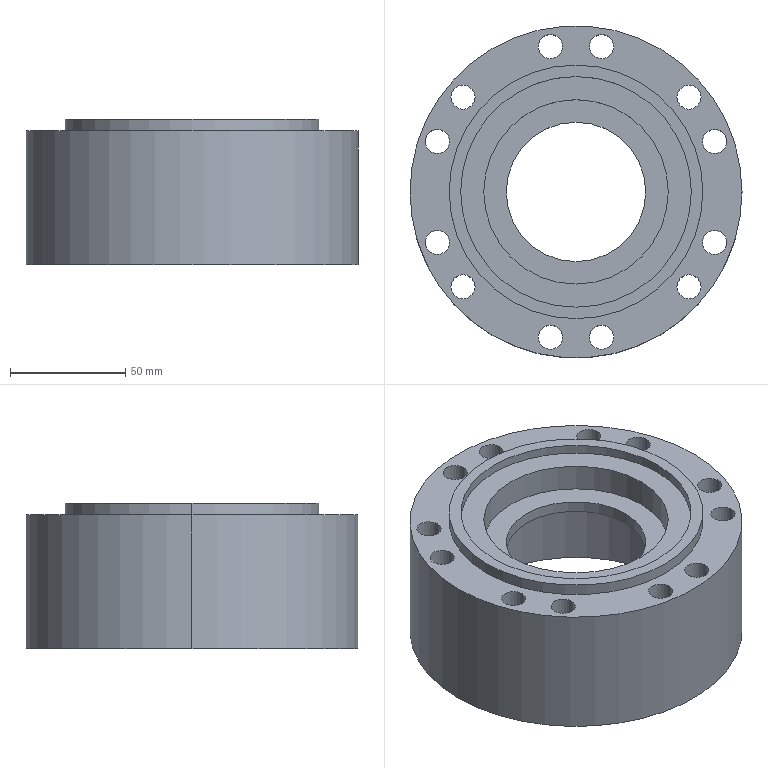Part | SolidWorks | features ICE 5, Extrusion 1, HoleWzd 1 | 1 solid | 42 faces | box 144 x 144 x 63 mm | volume 426591 mm3 | cylinder 36 | plane 6 | commonest cylinder face diameters 10.5 x24 110 x4 60.5 x2 80 x2 100 x2 144 x2
STEP:
#1=CARTESIAN_POINT('',(50.,0.,63.));
#2=VERTEX_POINT('',#1);
#3=CARTESIAN_POINT('',(-50.,0.,63.));
#4=VERTEX_POINT('',#3);
#5=CARTESIAN_POINT('',(0.,0.,63.));
#6=DIRECTION('',(0.,0.,-1.));
#7=DIRECTION('',(-1.,0.,0.));
#8=AXIS2_PLACEMENT_3D('',#5,#6,#7);
#9=CIRCLE('',#8,50.);
#10=EDGE_CURVE('',#2,#4,#9,.T.);
#11=ORIENTED_EDGE('',*,*,#10,.F.);
#12=CARTESIAN_POINT('',(50.,0.,59.));
#13=VERTEX_POINT('',#12);
#14=CARTESIAN_POINT('',(50.,0.,63.));
#15=DIRECTION('',(0.,0.,-1.));
#16=VECTOR('',#15,1000.);
#17=LINE('',#14,#16);
#18=EDGE_CURVE('',#2,#13,#17,.T.);
#19=ORIENTED_EDGE('',*,*,#18,.T.);
#20=CARTESIAN_POINT('',(-50.,0.,59.));
#21=VERTEX_POINT('',#20);
#22=CARTESIAN_POINT('',(0.,0.,59.));
#23=DIRECTION('',(0.,0.,-1.));
#24=DIRECTION('',(-1.,0.,0.));
#25=AXIS2_PLACEMENT_3D('',#22,#23,#24);
#26=CIRCLE('',#25,50.);
#27=EDGE_CURVE('',#13,#21,#26,.T.);
#28=ORIENTED_EDGE('',*,*,#27,.T.);
#29=CARTESIAN_POINT('',(-50.,0.,63.));
#30=DIRECTION('',(0.,0.,-1.));
#31=VECTOR('',#30,1000.);
#32=LINE('',#29,#31);
#33=EDGE_CURVE('',#4,#21,#32,.T.);
#34=ORIENTED_EDGE('',*,*,#33,.F.);
#35=EDGE_LOOP('',(#11,#19,#28,#34));
#36=FACE_OUTER_BOUND('',#35,.T.);
#37=CARTESIAN_POINT('',(0.,0.,63.));
#38=DIRECTION('',(0.,0.,-1.));
#39=DIRECTION('',(-1.,0.,0.));
#40=AXIS2_PLACEMENT_3D('',#37,#38,#39);
#41=CYLINDRICAL_SURFACE('',#40,50.);
#42=ADVANCED_FACE('',(#36),#41,.F.);
#43=CARTESIAN_POINT('',(-40.,0.,59.));
#44=VERTEX_POINT('',#43);
#45=CARTESIAN_POINT('',(40.,0.,59.));
#46=VERTEX_POINT('',#45);
#47=CARTESIAN_POINT('',(0.,0.,59.));
#48=DIRECTION('',(0.,0.,1.));
#49=DIRECTION('',(-1.,0.,0.));
#50=AXIS2_PLACEMENT_3D('',#47,#48,#49);
#51=CIRCLE('',#50,40.);
#52=EDGE_CURVE('',#44,#46,#51,.T.);
#53=ORIENTED_EDGE('',*,*,#52,.T.);
#54=CARTESIAN_POINT('',(40.,0.,47.));
#55=VERTEX_POINT('',#54);
#56=CARTESIAN_POINT('',(40.,0.,59.));
#57=DIRECTION('',(0.,0.,-1.));
#58=VECTOR('',#57,1000.);
#59=LINE('',#56,#58);
#60=EDGE_CURVE('',#46,#55,#59,.T.);
#61=ORIENTED_EDGE('',*,*,#60,.T.);
#62=CARTESIAN_POINT('',(-40.,0.,47.));
#63=VERTEX_POINT('',#62);
#64=CARTESIAN_POINT('',(0.,0.,47.));
#65=DIRECTION('',(0.,0.,-1.));
#66=DIRECTION('',(-1.,0.,0.));
#67=AXIS2_PLACEMENT_3D('',#64,#65,#66);
#68=CIRCLE('',#67,40.);
#69=EDGE_CURVE('',#55,#63,#68,.T.);
#70=ORIENTED_EDGE('',*,*,#69,.T.);
#71=CARTESIAN_POINT('',(-40.,0.,59.));
#72=DIRECTION('',(0.,0.,-1.));
#73=VECTOR('',#72,1000.);
#74=LINE('',#71,#73);
#75=EDGE_CURVE('',#44,#63,#74,.T.);
#76=ORIENTED_EDGE('',*,*,#75,.F.);
#77=EDGE_LOOP('',(#53,#61,#70,#76));
#78=FACE_OUTER_BOUND('',#77,.T.);
#79=CARTESIAN_POINT('',(0.,0.,59.));
#80=DIRECTION('',(0.,0.,-1.));
#81=DIRECTION('',(-1.,0.,0.));
#82=AXIS2_PLACEMENT_3D('',#79,#80,#81);
#83=CYLINDRICAL_SURFACE('',#82,40.);
#84=ADVANCED_FACE('',(#78),#83,.F.);
#85=CARTESIAN_POINT('',(-30.25,0.,47.));
#86=VERTEX_POINT('',#85);
#87=CARTESIAN_POINT('',(30.25,0.,47.));
#88=VERTEX_POINT('',#87);
#89=CARTESIAN_POINT('',(0.,0.,47.));
#90=DIRECTION('',(0.,0.,1.));
#91=DIRECTION('',(-1.,0.,0.));
#92=AXIS2_PLACEMENT_3D('',#89,#90,#91);
#93=CIRCLE('',#92,30.25);
#94=EDGE_CURVE('',#86,#88,#93,.T.);
#95=ORIENTED_EDGE('',*,*,#94,.T.);
#96=CARTESIAN_POINT('',(30.25,0.,42.));
#97=VERTEX_POINT('',#96);
#98=CARTESIAN_POINT('',(30.25,0.,47.));
#99=DIRECTION('',(0.,0.,-1.));
#100=VECTOR('',#99,1000.);
#101=LINE('',#98,#100);
#102=EDGE_CURVE('',#88,#97,#101,.T.);
#103=ORIENTED_EDGE('',*,*,#102,.T.);
#104=CARTESIAN_POINT('',(-30.25,0.,42.));
#105=VERTEX_POINT('',#104);
#106=CARTESIAN_POINT('',(0.,0.,42.));
#107=DIRECTION('',(0.,0.,-1.));
#108=DIRECTION('',(-1.,0.,0.));
#109=AXIS2_PLACEMENT_3D('',#106,#107,#108);
#110=CIRCLE('',#109,30.25);
#111=EDGE_CURVE('',#97,#105,#110,.T.);
#112=ORIENTED_EDGE('',*,*,#111,.T.);
#113=CARTESIAN_POINT('',(-30.25,0.,47.));
#114=DIRECTION('',(0.,0.,-1.));
#115=VECTOR('',#114,1000.);
#116=LINE('',#113,#115);
#117=EDGE_CURVE('',#86,#105,#116,.T.);
#118=ORIENTED_EDGE('',*,*,#117,.F.);
#119=EDGE_LOOP('',(#95,#103,#112,#118));
#120=FACE_OUTER_BOUND('',#119,.T.);
#121=CARTESIAN_POINT('',(0.,0.,47.));
#122=DIRECTION('',(0.,0.,-1.));
#123=DIRECTION('',(-1.,0.,0.));
#124=AXIS2_PLACEMENT_3D('',#121,#122,#123);
#125=CYLINDRICAL_SURFACE('',#124,30.25);
#126=ADVANCED_FACE('',(#120),#125,.F.);
#127=CARTESIAN_POINT('',(55.,0.,42.));
#128=VERTEX_POINT('',#127);
#129=CARTESIAN_POINT('',(-55.,0.,42.));
#130=VERTEX_POINT('',#129);
#131=CARTESIAN_POINT('',(0.,0.,42.));
#132=DIRECTION('',(0.,0.,-1.));
#133=DIRECTION('',(-1.,0.,0.));
#134=AXIS2_PLACEMENT_3D('',#131,#132,#133);
#135=CIRCLE('',#134,55.);
#136=EDGE_CURVE('',#128,#130,#135,.T.);
#137=ORIENTED_EDGE('',*,*,#136,.F.);
#138=CARTESIAN_POINT('',(55.,0.,0.));
#139=VERTEX_POINT('',#138);
#140=CARTESIAN_POINT('',(55.,0.,42.));
#141=DIRECTION('',(0.,0.,-1.));
#142=VECTOR('',#141,1000.);
#143=LINE('',#140,#142);
#144=EDGE_CURVE('',#128,#139,#143,.T.);
#145=ORIENTED_EDGE('',*,*,#144,.T.);
#146=CARTESIAN_POINT('',(-55.,0.,0.));
#147=VERTEX_POINT('',#146);
#148=CARTESIAN_POINT('',(0.,0.,0.));
#149=DIRECTION('',(0.,0.,-1.));
#150=DIRECTION('',(-1.,0.,0.));
#151=AXIS2_PLACEMENT_3D('',#148,#149,#150);
#152=CIRCLE('',#151,55.);
#153=EDGE_CURVE('',#139,#147,#152,.T.);
#154=ORIENTED_EDGE('',*,*,#153,.T.);
#155=CARTESIAN_POINT('',(-55.,0.,42.));
#156=DIRECTION('',(0.,0.,-1.));
#157=VECTOR('',#156,1000.);
#158=LINE('',#155,#157);
#159=EDGE_CURVE('',#130,#147,#158,.T.);
#160=ORIENTED_EDGE('',*,*,#159,.F.);
#161=EDGE_LOOP('',(#137,#145,#154,#160));
#162=FACE_OUTER_BOUND('',#161,.T.);
#163=CARTESIAN_POINT('',(0.,0.,42.));
#164=DIRECTION('',(0.,0.,-1.));
#165=DIRECTION('',(-1.,0.,0.));
#166=AXIS2_PLACEMENT_3D('',#163,#164,#165);
#167=CYLINDRICAL_SURFACE('',#166,55.);
#168=ADVANCED_FACE('',(#162),#167,.F.);
#169=CARTESIAN_POINT('',(5.863,63.028,58.));
#170=VERTEX_POINT('',#169);
#171=CARTESIAN_POINT('',(16.363,63.028,58.));
#172=VERTEX_POINT('',#171);
#173=CARTESIAN_POINT('',(11.113,63.028,58.));
#174=DIRECTION('',(0.,0.,1.));
#175=DIRECTION('',(1.,0.,0.));
#176=AXIS2_PLACEMENT_3D('',#173,#174,#175);
#177=CIRCLE('',#176,5.25);
#178=EDGE_CURVE('',#170,#172,#177,.T.);
#179=ORIENTED_EDGE('',*,*,#178,.T.);
#180=CARTESIAN_POINT('',(16.363,63.028,0.));
#181=VERTEX_POINT('',#180);
#182=CARTESIAN_POINT('',(16.363,63.028,0.));
#183=DIRECTION('',(0.,0.,-1.));
#184=VECTOR('',#183,1000.);
#185=LINE('',#182,#184);
#186=EDGE_CURVE('',#172,#181,#185,.T.);
#187=ORIENTED_EDGE('',*,*,#186,.T.);
#188=CARTESIAN_POINT('',(5.863,63.028,0.));
#189=VERTEX_POINT('',#188);
#190=CARTESIAN_POINT('',(11.113,63.028,0.));
#191=DIRECTION('',(0.,0.,-1.));
#192=DIRECTION('',(-1.,0.,0.));
#193=AXIS2_PLACEMENT_3D('',#190,#191,#192);
#194=CIRCLE('',#193,5.25);
#195=EDGE_CURVE('',#181,#189,#194,.T.);
#196=ORIENTED_EDGE('',*,*,#195,.T.);
#197=CARTESIAN_POINT('',(5.863,63.028,0.));
#198=DIRECTION('',(0.,0.,-1.));
#199=VECTOR('',#198,1000.);
#200=LINE('',#197,#199);
#201=EDGE_CURVE('',#170,#189,#200,.T.);
#202=ORIENTED_EDGE('',*,*,#201,.F.);
#203=EDGE_LOOP('',(#179,#187,#196,#202));
#204=FACE_OUTER_BOUND('',#203,.T.);
#205=CARTESIAN_POINT('',(11.113,63.028,0.));
#206=DIRECTION('',(0.,0.,-1.));
#207=DIRECTION('',(-1.,0.,0.));
#208=AXIS2_PLACEMENT_3D('',#205,#206,#207);
#209=CYLINDRICAL_SURFACE('',#208,5.25);
#210=ADVANCED_FACE('',(#204),#209,.F.);
#211=CARTESIAN_POINT('',(-16.363,63.028,58.));
#212=VERTEX_POINT('',#211);
#213=CARTESIAN_POINT('',(-5.863,63.028,58.));
#214=VERTEX_POINT('',#213);
#215=CARTESIAN_POINT('',(-11.113,63.028,58.));
#216=DIRECTION('',(0.,0.,1.));
#217=DIRECTION('',(1.,0.,0.));
#218=AXIS2_PLACEMENT_3D('',#215,#216,#217);
#219=CIRCLE('',#218,5.25);
#220=EDGE_CURVE('',#212,#214,#219,.T.);
#221=ORIENTED_EDGE('',*,*,#220,.T.);
#222=CARTESIAN_POINT('',(-5.863,63.028,0.));
#223=VERTEX_POINT('',#222);
#224=CARTESIAN_POINT('',(-5.863,63.028,0.));
#225=DIRECTION('',(0.,0.,-1.));
#226=VECTOR('',#225,1000.);
#227=LINE('',#224,#226);
#228=EDGE_CURVE('',#214,#223,#227,.T.);
#229=ORIENTED_EDGE('',*,*,#228,.T.);
#230=CARTESIAN_POINT('',(-16.363,63.028,0.));
#231=VERTEX_POINT('',#230);
#232=CARTESIAN_POINT('',(-11.113,63.028,0.));
#233=DIRECTION('',(0.,0.,-1.));
#234=DIRECTION('',(-1.,0.,0.));
#235=AXIS2_PLACEMENT_3D('',#232,#233,#234);
#236=CIRCLE('',#235,5.25);
#237=EDGE_CURVE('',#223,#231,#236,.T.);
#238=ORIENTED_EDGE('',*,*,#237,.T.);
#239=CARTESIAN_POINT('',(-16.363,63.028,0.));
#240=DIRECTION('',(0.,0.,-1.));
#241=VECTOR('',#240,1000.);
#242=LINE('',#239,#241);
#243=EDGE_CURVE('',#212,#231,#242,.T.);
#244=ORIENTED_EDGE('',*,*,#243,.F.);
#245=EDGE_LOOP('',(#221,#229,#238,#244));
#246=FACE_OUTER_BOUND('',#245,.T.);
#247=CARTESIAN_POINT('',(-11.113,63.028,0.));
#248=DIRECTION('',(0.,0.,-1.));
#249=DIRECTION('',(-1.,0.,0.));
#250=AXIS2_PLACEMENT_3D('',#247,#248,#249);
#251=CYLINDRICAL_SURFACE('',#250,5.25);
#252=ADVANCED_FACE('',(#246),#251,.F.);
#253=CARTESIAN_POINT('',(-54.277,41.138,58.));
#254=VERTEX_POINT('',#253);
#255=CARTESIAN_POINT('',(-43.777,41.138,58.));
#256=VERTEX_POINT('',#255);
#257=CARTESIAN_POINT('',(-49.027,41.138,58.));
#258=DIRECTION('',(0.,0.,1.));
#259=DIRECTION('',(1.,0.,0.));
#260=AXIS2_PLACEMENT_3D('',#257,#258,#259);
#261=CIRCLE('',#260,5.25);
#262=EDGE_CURVE('',#254,#256,#261,.T.);
#263=ORIENTED_EDGE('',*,*,#262,.T.);
#264=CARTESIAN_POINT('',(-43.777,41.138,0.));
#265=VERTEX_POINT('',#264);
#266=CARTESIAN_POINT('',(-43.777,41.138,0.));
#267=DIRECTION('',(0.,0.,-1.));
#268=VECTOR('',#267,1000.);
#269=LINE('',#266,#268);
#270=EDGE_CURVE('',#256,#265,#269,.T.);
#271=ORIENTED_EDGE('',*,*,#270,.T.);
#272=CARTESIAN_POINT('',(-54.277,41.138,0.));
#273=VERTEX_POINT('',#272);
#274=CARTESIAN_POINT('',(-49.027,41.138,0.));
#275=DIRECTION('',(0.,0.,-1.));
#276=DIRECTION('',(-1.,0.,0.));
#277=AXIS2_PLACEMENT_3D('',#274,#275,#276);
#278=CIRCLE('',#277,5.25);
#279=EDGE_CURVE('',#265,#273,#278,.T.);
#280=ORIENTED_EDGE('',*,*,#279,.T.);
#281=CARTESIAN_POINT('',(-54.277,41.138,0.));
#282=DIRECTION('',(0.,0.,-1.));
#283=VECTOR('',#282,1000.);
#284=LINE('',#281,#283);
#285=EDGE_CURVE('',#254,#273,#284,.T.);
#286=ORIENTED_EDGE('',*,*,#285,.F.);
#287=EDGE_LOOP('',(#263,#271,#280,#286));
#288=FACE_OUTER_BOUND('',#287,.T.);
#289=CARTESIAN_POINT('',(-49.027,41.138,0.));
#290=DIRECTION('',(0.,0.,-1.));
#291=DIRECTION('',(-1.,0.,0.));
#292=AXIS2_PLACEMENT_3D('',#289,#290,#291);
#293=CYLINDRICAL_SURFACE('',#292,5.25);
#294=ADVANCED_FACE('',(#288),#293,.F.);
#295=CARTESIAN_POINT('',(-65.39,21.889,58.));
#296=VERTEX_POINT('',#295);
#297=CARTESIAN_POINT('',(-54.89,21.889,58.));
#298=VERTEX_POINT('',#297);
#299=CARTESIAN_POINT('',(-60.14,21.889,58.));
#300=DIRECTION('',(0.,0.,1.));
#301=DIRECTION('',(1.,0.,0.));
#302=AXIS2_PLACEMENT_3D('',#299,#300,#301);
#303=CIRCLE('',#302,5.25);
#304=EDGE_CURVE('',#296,#298,#303,.T.);
#305=ORIENTED_EDGE('',*,*,#304,.T.);
#306=CARTESIAN_POINT('',(-54.89,21.889,0.));
#307=VERTEX_POINT('',#306);
#308=CARTESIAN_POINT('',(-54.89,21.889,0.));
#309=DIRECTION('',(0.,0.,-1.));
#310=VECTOR('',#309,1000.);
#311=LINE('',#308,#310);
#312=EDGE_CURVE('',#298,#307,#311,.T.);
#313=ORIENTED_EDGE('',*,*,#312,.T.);
#314=CARTESIAN_POINT('',(-65.39,21.889,0.));
#315=VERTEX_POINT('',#314);
#316=CARTESIAN_POINT('',(-60.14,21.889,0.));
#317=DIRECTION('',(0.,0.,-1.));
#318=DIRECTION('',(-1.,0.,0.));
#319=AXIS2_PLACEMENT_3D('',#316,#317,#318);
#320=CIRCLE('',#319,5.25);
#321=EDGE_CURVE('',#307,#315,#320,.T.);
#322=ORIENTED_EDGE('',*,*,#321,.T.);
#323=CARTESIAN_POINT('',(-65.39,21.889,0.));
#324=DIRECTION('',(0.,0.,-1.));
#325=VECTOR('',#324,1000.);
#326=LINE('',#323,#325);
#327=EDGE_CURVE('',#296,#315,#326,.T.);
#328=ORIENTED_EDGE('',*,*,#327,.F.);
#329=EDGE_LOOP('',(#305,#313,#322,#328));
#330=FACE_OUTER_BOUND('',#329,.T.);
#331=CARTESIAN_POINT('',(-60.14,21.889,0.));
#332=DIRECTION('',(0.,0.,-1.));
#333=DIRECTION('',(-1.,0.,0.));
#334=AXIS2_PLACEMENT_3D('',#331,#332,#333);
#335=CYLINDRICAL_SURFACE('',#334,5.25);
#336=ADVANCED_FACE('',(#330),#335,.F.);
#337=CARTESIAN_POINT('',(-65.39,-21.889,58.));
#338=VERTEX_POINT('',#337);
#339=CARTESIAN_POINT('',(-54.89,-21.889,58.));
#340=VERTEX_POINT('',#339);
#341=CARTESIAN_POINT('',(-60.14,-21.889,58.));
#342=DIRECTION('',(0.,0.,1.));
#343=DIRECTION('',(1.,0.,0.));
#344=AXIS2_PLACEMENT_3D('',#341,#342,#343);
#345=CIRCLE('',#344,5.25);
#346=EDGE_CURVE('',#338,#340,#345,.T.);
#347=ORIENTED_EDGE('',*,*,#346,.T.);
#348=CARTESIAN_POINT('',(-54.89,-21.889,0.));
#349=VERTEX_POINT('',#348);
#350=CARTESIAN_POINT('',(-54.89,-21.889,0.));
#351=DIRECTION('',(0.,0.,-1.));
#352=VECTOR('',#351,1000.);
#353=LINE('',#350,#352);
#354=EDGE_CURVE('',#340,#349,#353,.T.);
#355=ORIENTED_EDGE('',*,*,#354,.T.);
#356=CARTESIAN_POINT('',(-65.39,-21.889,0.));
#357=VERTEX_POINT('',#356);
#358=CARTESIAN_POINT('',(-60.14,-21.889,0.));
#359=DIRECTION('',(0.,0.,-1.));
#360=DIRECTION('',(-1.,0.,0.));
#361=AXIS2_PLACEMENT_3D('',#358,#359,#360);
#362=CIRCLE('',#361,5.25);
#363=EDGE_CURVE('',#349,#357,#362,.T.);
#364=ORIENTED_EDGE('',*,*,#363,.T.);
#365=CARTESIAN_POINT('',(-65.39,-21.889,0.));
#366=DIRECTION('',(0.,0.,-1.));
#367=VECTOR('',#366,1000.);
#368=LINE('',#365,#367);
#369=EDGE_CURVE('',#338,#357,#368,.T.);
#370=ORIENTED_EDGE('',*,*,#369,.F.);
#371=EDGE_LOOP('',(#347,#355,#364,#370));
#372=FACE_OUTER_BOUND('',#371,.T.);
#373=CARTESIAN_POINT('',(-60.14,-21.889,0.));
#374=DIRECTION('',(0.,0.,-1.));
#375=DIRECTION('',(-1.,0.,0.));
#376=AXIS2_PLACEMENT_3D('',#373,#374,#375);
#377=CYLINDRICAL_SURFACE('',#376,5.25);
#378=ADVANCED_FACE('',(#372),#377,.F.);
#379=CARTESIAN_POINT('',(-54.277,-41.138,58.));
#380=VERTEX_POINT('',#379);
#381=CARTESIAN_POINT('',(-43.777,-41.138,58.));
#382=VERTEX_POINT('',#381);
#383=CARTESIAN_POINT('',(-49.027,-41.138,58.));
#384=DIRECTION('',(0.,0.,1.));
#385=DIRECTION('',(1.,0.,0.));
#386=AXIS2_PLACEMENT_3D('',#383,#384,#385);
#387=CIRCLE('',#386,5.25);
#388=EDGE_CURVE('',#380,#382,#387,.T.);
#389=ORIENTED_EDGE('',*,*,#388,.T.);
#390=CARTESIAN_POINT('',(-43.777,-41.138,0.));
#391=VERTEX_POINT('',#390);
#392=CARTESIAN_POINT('',(-43.777,-41.138,0.));
#393=DIRECTION('',(0.,0.,-1.));
#394=VECTOR('',#393,1000.);
#395=LINE('',#392,#394);
#396=EDGE_CURVE('',#382,#391,#395,.T.);
#397=ORIENTED_EDGE('',*,*,#396,.T.);
#398=CARTESIAN_POINT('',(-54.277,-41.138,0.));
#399=VERTEX_POINT('',#398);
#400=CARTESIAN_POINT('',(-49.027,-41.138,0.));
#401=DIRECTION('',(0.,0.,-1.));
#402=DIRECTION('',(-1.,0.,0.));
#403=AXIS2_PLACEMENT_3D('',#400,#401,#402);
#404=CIRCLE('',#403,5.25);
#405=EDGE_CURVE('',#391,#399,#404,.T.);
#406=ORIENTED_EDGE('',*,*,#405,.T.);
#407=CARTESIAN_POINT('',(-54.277,-41.138,0.));
#408=DIRECTION('',(0.,0.,-1.));
#409=VECTOR('',#408,1000.);
#410=LINE('',#407,#409);
#411=EDGE_CURVE('',#380,#399,#410,.T.);
#412=ORIENTED_EDGE('',*,*,#411,.F.);
#413=EDGE_LOOP('',(#389,#397,#406,#412));
#414=FACE_OUTER_BOUND('',#413,.T.);
#415=CARTESIAN_POINT('',(-49.027,-41.138,0.));
#416=DIRECTION('',(0.,0.,-1.));
#417=DIRECTION('',(-1.,0.,0.));
#418=AXIS2_PLACEMENT_3D('',#415,#416,#417);
#419=CYLINDRICAL_SURFACE('',#418,5.25);
#420=ADVANCED_FACE('',(#414),#419,.F.);
#421=CARTESIAN_POINT('',(-16.363,-63.028,58.));
#422=VERTEX_POINT('',#421);
#423=CARTESIAN_POINT('',(-5.863,-63.028,58.));
#424=VERTEX_POINT('',#423);
#425=CARTESIAN_POINT('',(-11.113,-63.028,58.));
#426=DIRECTION('',(0.,0.,1.));
#427=DIRECTION('',(1.,0.,0.));
#428=AXIS2_PLACEMENT_3D('',#425,#426,#427);
#429=CIRCLE('',#428,5.25);
#430=EDGE_CURVE('',#422,#424,#429,.T.);
#431=ORIENTED_EDGE('',*,*,#430,.T.);
#432=CARTESIAN_POINT('',(-5.863,-63.028,0.));
#433=VERTEX_POINT('',#432);
#434=CARTESIAN_POINT('',(-5.863,-63.028,0.));
#435=DIRECTION('',(0.,0.,-1.));
#436=VECTOR('',#435,1000.);
#437=LINE('',#434,#436);
#438=EDGE_CURVE('',#424,#433,#437,.T.);
#439=ORIENTED_EDGE('',*,*,#438,.T.);
#440=CARTESIAN_POINT('',(-16.363,-63.028,0.));
#441=VERTEX_POINT('',#440);
#442=CARTESIAN_POINT('',(-11.113,-63.028,0.));
#443=DIRECTION('',(0.,0.,-1.));
#444=DIRECTION('',(-1.,0.,0.));
#445=AXIS2_PLACEMENT_3D('',#442,#443,#444);
#446=CIRCLE('',#445,5.25);
#447=EDGE_CURVE('',#433,#441,#446,.T.);
#448=ORIENTED_EDGE('',*,*,#447,.T.);
#449=CARTESIAN_POINT('',(-16.363,-63.028,0.));
#450=DIRECTION('',(0.,0.,-1.));
#451=VECTOR('',#450,1000.);
#452=LINE('',#449,#451);
#453=EDGE_CURVE('',#422,#441,#452,.T.);
#454=ORIENTED_EDGE('',*,*,#453,.F.);
#455=EDGE_LOOP('',(#431,#439,#448,#454));
#456=FACE_OUTER_BOUND('',#455,.T.);
#457=CARTESIAN_POINT('',(-11.113,-63.028,0.));
#458=DIRECTION('',(0.,0.,-1.));
#459=DIRECTION('',(-1.,0.,0.));
#460=AXIS2_PLACEMENT_3D('',#457,#458,#459);
#461=CYLINDRICAL_SURFACE('',#460,5.25);
#462=ADVANCED_FACE('',(#456),#461,.F.);
#463=CARTESIAN_POINT('',(5.863,-63.028,58.));
#464=VERTEX_POINT('',#463);
#465=CARTESIAN_POINT('',(16.363,-63.028,58.));
#466=VERTEX_POINT('',#465);
#467=CARTESIAN_POINT('',(11.113,-63.028,58.));
#468=DIRECTION('',(0.,0.,1.));
#469=DIRECTION('',(1.,0.,0.));
#470=AXIS2_PLACEMENT_3D('',#467,#468,#469);
#471=CIRCLE('',#470,5.25);
#472=EDGE_CURVE('',#464,#466,#471,.T.);
#473=ORIENTED_EDGE('',*,*,#472,.T.);
#474=CARTESIAN_POINT('',(16.363,-63.028,0.));
#475=VERTEX_POINT('',#474);
#476=CARTESIAN_POINT('',(16.363,-63.028,0.));
#477=DIRECTION('',(0.,0.,-1.));
#478=VECTOR('',#477,1000.);
#479=LINE('',#476,#478);
#480=EDGE_CURVE('',#466,#475,#479,.T.);
#481=ORIENTED_EDGE('',*,*,#480,.T.);
#482=CARTESIAN_POINT('',(5.863,-63.028,0.));
#483=VERTEX_POINT('',#482);
#484=CARTESIAN_POINT('',(11.113,-63.028,0.));
#485=DIRECTION('',(0.,0.,-1.));
#486=DIRECTION('',(-1.,0.,0.));
#487=AXIS2_PLACEMENT_3D('',#484,#485,#486);
#488=CIRCLE('',#487,5.25);
#489=EDGE_CURVE('',#475,#483,#488,.T.);
#490=ORIENTED_EDGE('',*,*,#489,.T.);
#491=CARTESIAN_POINT('',(5.863,-63.028,0.));
#492=DIRECTION('',(0.,0.,-1.));
#493=VECTOR('',#492,1000.);
#494=LINE('',#491,#493);
#495=EDGE_CURVE('',#464,#483,#494,.T.);
#496=ORIENTED_EDGE('',*,*,#495,.F.);
#497=EDGE_LOOP('',(#473,#481,#490,#496));
#498=FACE_OUTER_BOUND('',#497,.T.);
#499=CARTESIAN_POINT('',(11.113,-63.028,0.));
#500=DIRECTION('',(0.,0.,-1.));
#501=DIRECTION('',(-1.,0.,0.));
#502=AXIS2_PLACEMENT_3D('',#499,#500,#501);
#503=CYLINDRICAL_SURFACE('',#502,5.25);
#504=ADVANCED_FACE('',(#498),#503,.F.);
#505=CARTESIAN_POINT('',(43.777,-41.138,58.));
#506=VERTEX_POINT('',#505);
#507=CARTESIAN_POINT('',(54.277,-41.138,58.));
#508=VERTEX_POINT('',#507);
#509=CARTESIAN_POINT('',(49.027,-41.138,58.));
#510=DIRECTION('',(0.,0.,1.));
#511=DIRECTION('',(1.,0.,0.));
#512=AXIS2_PLACEMENT_3D('',#509,#510,#511);
#513=CIRCLE('',#512,5.25);
#514=EDGE_CURVE('',#506,#508,#513,.T.);
#515=ORIENTED_EDGE('',*,*,#514,.T.);
#516=CARTESIAN_POINT('',(54.277,-41.138,0.));
#517=VERTEX_POINT('',#516);
#518=CARTESIAN_POINT('',(54.277,-41.138,0.));
#519=DIRECTION('',(0.,0.,-1.));
#520=VECTOR('',#519,1000.);
#521=LINE('',#518,#520);
#522=EDGE_CURVE('',#508,#517,#521,.T.);
#523=ORIENTED_EDGE('',*,*,#522,.T.);
#524=CARTESIAN_POINT('',(43.777,-41.138,0.));
#525=VERTEX_POINT('',#524);
#526=CARTESIAN_POINT('',(49.027,-41.138,0.));
#527=DIRECTION('',(0.,0.,-1.));
#528=DIRECTION('',(-1.,0.,0.));
#529=AXIS2_PLACEMENT_3D('',#526,#527,#528);
#530=CIRCLE('',#529,5.25);
#531=EDGE_CURVE('',#517,#525,#530,.T.);
#532=ORIENTED_EDGE('',*,*,#531,.T.);
#533=CARTESIAN_POINT('',(43.777,-41.138,0.));
#534=DIRECTION('',(0.,0.,-1.));
#535=VECTOR('',#534,1000.);
#536=LINE('',#533,#535);
#537=EDGE_CURVE('',#506,#525,#536,.T.);
#538=ORIENTED_EDGE('',*,*,#537,.F.);
#539=EDGE_LOOP('',(#515,#523,#532,#538));
#540=FACE_OUTER_BOUND('',#539,.T.);
#541=CARTESIAN_POINT('',(49.027,-41.138,0.));
#542=DIRECTION('',(0.,0.,-1.));
#543=DIRECTION('',(-1.,0.,0.));
#544=AXIS2_PLACEMENT_3D('',#541,#542,#543);
#545=CYLINDRICAL_SURFACE('',#544,5.25);
#546=ADVANCED_FACE('',(#540),#545,.F.);
#547=CARTESIAN_POINT('',(54.89,-21.889,58.));
#548=VERTEX_POINT('',#547);
#549=CARTESIAN_POINT('',(65.39,-21.889,58.));
#550=VERTEX_POINT('',#549);
#551=CARTESIAN_POINT('',(60.14,-21.889,58.));
#552=DIRECTION('',(0.,0.,1.));
#553=DIRECTION('',(1.,0.,0.));
#554=AXIS2_PLACEMENT_3D('',#551,#552,#553);
#555=CIRCLE('',#554,5.25);
#556=EDGE_CURVE('',#548,#550,#555,.T.);
#557=ORIENTED_EDGE('',*,*,#556,.T.);
#558=CARTESIAN_POINT('',(65.39,-21.889,0.));
#559=VERTEX_POINT('',#558);
#560=CARTESIAN_POINT('',(65.39,-21.889,0.));
#561=DIRECTION('',(0.,0.,-1.));
#562=VECTOR('',#561,1000.);
#563=LINE('',#560,#562);
#564=EDGE_CURVE('',#550,#559,#563,.T.);
#565=ORIENTED_EDGE('',*,*,#564,.T.);
#566=CARTESIAN_POINT('',(54.89,-21.889,0.));
#567=VERTEX_POINT('',#566);
#568=CARTESIAN_POINT('',(60.14,-21.889,0.));
#569=DIRECTION('',(0.,0.,-1.));
#570=DIRECTION('',(-1.,0.,0.));
#571=AXIS2_PLACEMENT_3D('',#568,#569,#570);
#572=CIRCLE('',#571,5.25);
#573=EDGE_CURVE('',#559,#567,#572,.T.);
#574=ORIENTED_EDGE('',*,*,#573,.T.);
#575=CARTESIAN_POINT('',(54.89,-21.889,0.));
#576=DIRECTION('',(0.,0.,-1.));
#577=VECTOR('',#576,1000.);
#578=LINE('',#575,#577);
#579=EDGE_CURVE('',#548,#567,#578,.T.);
#580=ORIENTED_EDGE('',*,*,#579,.F.);
#581=EDGE_LOOP('',(#557,#565,#574,#580));
#582=FACE_OUTER_BOUND('',#581,.T.);
#583=CARTESIAN_POINT('',(60.14,-21.889,0.));
#584=DIRECTION('',(0.,0.,-1.));
#585=DIRECTION('',(-1.,0.,0.));
#586=AXIS2_PLACEMENT_3D('',#583,#584,#585);
#587=CYLINDRICAL_SURFACE('',#586,5.25);
#588=ADVANCED_FACE('',(#582),#587,.F.);
#589=CARTESIAN_POINT('',(54.89,21.889,58.));
#590=VERTEX_POINT('',#589);
#591=CARTESIAN_POINT('',(65.39,21.889,58.));
#592=VERTEX_POINT('',#591);
#593=CARTESIAN_POINT('',(60.14,21.889,58.));
#594=DIRECTION('',(0.,0.,1.));
#595=DIRECTION('',(1.,0.,0.));
#596=AXIS2_PLACEMENT_3D('',#593,#594,#595);
#597=CIRCLE('',#596,5.25);
#598=EDGE_CURVE('',#590,#592,#597,.T.);
#599=ORIENTED_EDGE('',*,*,#598,.T.);
#600=CARTESIAN_POINT('',(65.39,21.889,0.));
#601=VERTEX_POINT('',#600);
#602=CARTESIAN_POINT('',(65.39,21.889,0.));
#603=DIRECTION('',(0.,0.,-1.));
#604=VECTOR('',#603,1000.);
#605=LINE('',#602,#604);
#606=EDGE_CURVE('',#592,#601,#605,.T.);
#607=ORIENTED_EDGE('',*,*,#606,.T.);
#608=CARTESIAN_POINT('',(54.89,21.889,0.));
#609=VERTEX_POINT('',#608);
#610=CARTESIAN_POINT('',(60.14,21.889,0.));
#611=DIRECTION('',(0.,0.,-1.));
#612=DIRECTION('',(-1.,0.,0.));
#613=AXIS2_PLACEMENT_3D('',#610,#611,#612);
#614=CIRCLE('',#613,5.25);
#615=EDGE_CURVE('',#601,#609,#614,.T.);
#616=ORIENTED_EDGE('',*,*,#615,.T.);
#617=CARTESIAN_POINT('',(54.89,21.889,0.));
#618=DIRECTION('',(0.,0.,-1.));
#619=VECTOR('',#618,1000.);
#620=LINE('',#617,#619);
#621=EDGE_CURVE('',#590,#609,#620,.T.);
#622=ORIENTED_EDGE('',*,*,#621,.F.);
#623=EDGE_LOOP('',(#599,#607,#616,#622));
#624=FACE_OUTER_BOUND('',#623,.T.);
#625=CARTESIAN_POINT('',(60.14,21.889,0.));
#626=DIRECTION('',(0.,0.,-1.));
#627=DIRECTION('',(-1.,0.,0.));
#628=AXIS2_PLACEMENT_3D('',#625,#626,#627);
#629=CYLINDRICAL_SURFACE('',#628,5.25);
#630=ADVANCED_FACE('',(#624),#629,.F.);
#631=CARTESIAN_POINT('',(43.777,41.138,58.));
#632=VERTEX_POINT('',#631);
#633=CARTESIAN_POINT('',(54.277,41.138,58.));
#634=VERTEX_POINT('',#633);
#635=CARTESIAN_POINT('',(49.027,41.138,58.));
#636=DIRECTION('',(0.,0.,1.));
#637=DIRECTION('',(1.,0.,0.));
#638=AXIS2_PLACEMENT_3D('',#635,#636,#637);
#639=CIRCLE('',#638,5.25);
#640=EDGE_CURVE('',#632,#634,#639,.T.);
#641=ORIENTED_EDGE('',*,*,#640,.T.);
#642=CARTESIAN_POINT('',(54.277,41.138,0.));
#643=VERTEX_POINT('',#642);
#644=CARTESIAN_POINT('',(54.277,41.138,0.));
#645=DIRECTION('',(0.,0.,-1.));
#646=VECTOR('',#645,1000.);
#647=LINE('',#644,#646);
#648=EDGE_CURVE('',#634,#643,#647,.T.);
#649=ORIENTED_EDGE('',*,*,#648,.T.);
#650=CARTESIAN_POINT('',(43.777,41.138,0.));
#651=VERTEX_POINT('',#650);
#652=CARTESIAN_POINT('',(49.027,41.138,0.));
#653=DIRECTION('',(0.,0.,-1.));
#654=DIRECTION('',(-1.,0.,0.));
#655=AXIS2_PLACEMENT_3D('',#652,#653,#654);
#656=CIRCLE('',#655,5.25);
#657=EDGE_CURVE('',#643,#651,#656,.T.);
#658=ORIENTED_EDGE('',*,*,#657,.T.);
#659=CARTESIAN_POINT('',(43.777,41.138,0.));
#660=DIRECTION('',(0.,0.,-1.));
#661=VECTOR('',#660,1000.);
#662=LINE('',#659,#661);
#663=EDGE_CURVE('',#632,#651,#662,.T.);
#664=ORIENTED_EDGE('',*,*,#663,.F.);
#665=EDGE_LOOP('',(#641,#649,#658,#664));
#666=FACE_OUTER_BOUND('',#665,.T.);
#667=CARTESIAN_POINT('',(49.027,41.138,0.));
#668=DIRECTION('',(0.,0.,-1.));
#669=DIRECTION('',(-1.,0.,0.));
#670=AXIS2_PLACEMENT_3D('',#667,#668,#669);
#671=CYLINDRICAL_SURFACE('',#670,5.25);
#672=ADVANCED_FACE('',(#666),#671,.F.);
#673=CARTESIAN_POINT('',(55.,0.,63.));
#674=VERTEX_POINT('',#673);
#675=CARTESIAN_POINT('',(-55.,0.,63.));
#676=VERTEX_POINT('',#675);
#677=CARTESIAN_POINT('',(0.,0.,63.));
#678=DIRECTION('',(0.,0.,1.));
#679=DIRECTION('',(1.,0.,0.));
#680=AXIS2_PLACEMENT_3D('',#677,#678,#679);
#681=CIRCLE('',#680,55.);
#682=EDGE_CURVE('',#674,#676,#681,.T.);
#683=ORIENTED_EDGE('',*,*,#682,.F.);
#684=CARTESIAN_POINT('',(55.,0.,58.));
#685=VERTEX_POINT('',#684);
#686=CARTESIAN_POINT('',(55.,0.,63.));
#687=DIRECTION('',(0.,0.,-1.));
#688=VECTOR('',#687,1000.);
#689=LINE('',#686,#688);
#690=EDGE_CURVE('',#674,#685,#689,.T.);
#691=ORIENTED_EDGE('',*,*,#690,.T.);
#692=CARTESIAN_POINT('',(-55.,0.,58.));
#693=VERTEX_POINT('',#692);
#694=CARTESIAN_POINT('',(0.,0.,58.));
#695=DIRECTION('',(0.,0.,1.));
#696=DIRECTION('',(1.,0.,0.));
#697=AXIS2_PLACEMENT_3D('',#694,#695,#696);
#698=CIRCLE('',#697,55.);
#699=EDGE_CURVE('',#685,#693,#698,.T.);
#700=ORIENTED_EDGE('',*,*,#699,.T.);
#701=CARTESIAN_POINT('',(-55.,0.,63.));
#702=DIRECTION('',(0.,0.,-1.));
#703=VECTOR('',#702,1000.);
#704=LINE('',#701,#703);
#705=EDGE_CURVE('',#676,#693,#704,.T.);
#706=ORIENTED_EDGE('',*,*,#705,.F.);
#707=EDGE_LOOP('',(#683,#691,#700,#706));
#708=FACE_OUTER_BOUND('',#707,.T.);
#709=CARTESIAN_POINT('',(0.,0.,63.));
#710=DIRECTION('',(0.,0.,-1.));
#711=DIRECTION('',(-1.,0.,0.));
#712=AXIS2_PLACEMENT_3D('',#709,#710,#711);
#713=CYLINDRICAL_SURFACE('',#712,55.);
#714=ADVANCED_FACE('',(#708),#713,.T.);
#715=CARTESIAN_POINT('',(72.,0.,58.));
#716=VERTEX_POINT('',#715);
#717=CARTESIAN_POINT('',(-72.,0.,58.));
#718=VERTEX_POINT('',#717);
#719=CARTESIAN_POINT('',(0.,0.,58.));
#720=DIRECTION('',(0.,0.,1.));
#721=DIRECTION('',(1.,0.,0.));
#722=AXIS2_PLACEMENT_3D('',#719,#720,#721);
#723=CIRCLE('',#722,72.);
#724=EDGE_CURVE('',#716,#718,#723,.T.);
#725=ORIENTED_EDGE('',*,*,#724,.F.);
#726=CARTESIAN_POINT('',(72.,0.,0.));
#727=VERTEX_POINT('',#726);
#728=CARTESIAN_POINT('',(72.,0.,58.));
#729=DIRECTION('',(0.,0.,-1.));
#730=VECTOR('',#729,1000.);
#731=LINE('',#728,#730);
#732=EDGE_CURVE('',#716,#727,#731,.T.);
#733=ORIENTED_EDGE('',*,*,#732,.T.);
#734=CARTESIAN_POINT('',(-72.,0.,0.));
#735=VERTEX_POINT('',#734);
#736=CARTESIAN_POINT('',(0.,0.,0.));
#737=DIRECTION('',(0.,0.,1.));
#738=DIRECTION('',(1.,0.,0.));
#739=AXIS2_PLACEMENT_3D('',#736,#737,#738);
#740=CIRCLE('',#739,72.);
#741=EDGE_CURVE('',#727,#735,#740,.T.);
#742=ORIENTED_EDGE('',*,*,#741,.T.);
#743=CARTESIAN_POINT('',(-72.,0.,58.));
#744=DIRECTION('',(0.,0.,-1.));
#745=VECTOR('',#744,1000.);
#746=LINE('',#743,#745);
#747=EDGE_CURVE('',#718,#735,#746,.T.);
#748=ORIENTED_EDGE('',*,*,#747,.F.);
#749=EDGE_LOOP('',(#725,#733,#742,#748));
#750=FACE_OUTER_BOUND('',#749,.T.);
#751=CARTESIAN_POINT('',(0.,0.,58.));
#752=DIRECTION('',(0.,0.,-1.));
#753=DIRECTION('',(-1.,0.,0.));
#754=AXIS2_PLACEMENT_3D('',#751,#752,#753);
#755=CYLINDRICAL_SURFACE('',#754,72.);
#756=ADVANCED_FACE('',(#750),#755,.T.);
#757=ORIENTED_EDGE('',*,*,#178,.F.);
#758=CARTESIAN_POINT('',(11.113,63.028,58.));
#759=DIRECTION('',(0.,0.,1.));
#760=DIRECTION('',(1.,0.,0.));
#761=AXIS2_PLACEMENT_3D('',#758,#759,#760);
#762=CIRCLE('',#761,5.25);
#763=EDGE_CURVE('',#172,#170,#762,.T.);
#764=ORIENTED_EDGE('',*,*,#763,.F.);
#765=EDGE_LOOP('',(#757,#764));
#766=FACE_BOUND('',#765,.T.);
#767=ORIENTED_EDGE('',*,*,#220,.F.);
#768=CARTESIAN_POINT('',(-11.113,63.028,58.));
#769=DIRECTION('',(0.,0.,1.));
#770=DIRECTION('',(1.,0.,0.));
#771=AXIS2_PLACEMENT_3D('',#768,#769,#770);
#772=CIRCLE('',#771,5.25);
#773=EDGE_CURVE('',#214,#212,#772,.T.);
#774=ORIENTED_EDGE('',*,*,#773,.F.);
#775=EDGE_LOOP('',(#767,#774));
#776=FACE_BOUND('',#775,.T.);
#777=ORIENTED_EDGE('',*,*,#262,.F.);
#778=CARTESIAN_POINT('',(-49.027,41.138,58.));
#779=DIRECTION('',(0.,0.,1.));
#780=DIRECTION('',(1.,0.,0.));
#781=AXIS2_PLACEMENT_3D('',#778,#779,#780);
#782=CIRCLE('',#781,5.25);
#783=EDGE_CURVE('',#256,#254,#782,.T.);
#784=ORIENTED_EDGE('',*,*,#783,.F.);
#785=EDGE_LOOP('',(#777,#784));
#786=FACE_BOUND('',#785,.T.);
#787=ORIENTED_EDGE('',*,*,#304,.F.);
#788=CARTESIAN_POINT('',(-60.14,21.889,58.));
#789=DIRECTION('',(0.,0.,1.));
#790=DIRECTION('',(1.,0.,0.));
#791=AXIS2_PLACEMENT_3D('',#788,#789,#790);
#792=CIRCLE('',#791,5.25);
#793=EDGE_CURVE('',#298,#296,#792,.T.);
#794=ORIENTED_EDGE('',*,*,#793,.F.);
#795=EDGE_LOOP('',(#787,#794));
#796=FACE_BOUND('',#795,.T.);
#797=ORIENTED_EDGE('',*,*,#346,.F.);
#798=CARTESIAN_POINT('',(-60.14,-21.889,58.));
#799=DIRECTION('',(0.,0.,1.));
#800=DIRECTION('',(1.,0.,0.));
#801=AXIS2_PLACEMENT_3D('',#798,#799,#800);
#802=CIRCLE('',#801,5.25);
#803=EDGE_CURVE('',#340,#338,#802,.T.);
#804=ORIENTED_EDGE('',*,*,#803,.F.);
#805=EDGE_LOOP('',(#797,#804));
#806=FACE_BOUND('',#805,.T.);
#807=ORIENTED_EDGE('',*,*,#388,.F.);
#808=CARTESIAN_POINT('',(-49.027,-41.138,58.));
#809=DIRECTION('',(0.,0.,1.));
#810=DIRECTION('',(1.,0.,0.));
#811=AXIS2_PLACEMENT_3D('',#808,#809,#810);
#812=CIRCLE('',#811,5.25);
#813=EDGE_CURVE('',#382,#380,#812,.T.);
#814=ORIENTED_EDGE('',*,*,#813,.F.);
#815=EDGE_LOOP('',(#807,#814));
#816=FACE_BOUND('',#815,.T.);
#817=ORIENTED_EDGE('',*,*,#430,.F.);
#818=CARTESIAN_POINT('',(-11.113,-63.028,58.));
#819=DIRECTION('',(0.,0.,1.));
#820=DIRECTION('',(1.,0.,0.));
#821=AXIS2_PLACEMENT_3D('',#818,#819,#820);
#822=CIRCLE('',#821,5.25);
#823=EDGE_CURVE('',#424,#422,#822,.T.);
#824=ORIENTED_EDGE('',*,*,#823,.F.);
#825=EDGE_LOOP('',(#817,#824));
#826=FACE_BOUND('',#825,.T.);
#827=ORIENTED_EDGE('',*,*,#472,.F.);
#828=CARTESIAN_POINT('',(11.113,-63.028,58.));
#829=DIRECTION('',(0.,0.,1.));
#830=DIRECTION('',(1.,0.,0.));
#831=AXIS2_PLACEMENT_3D('',#828,#829,#830);
#832=CIRCLE('',#831,5.25);
#833=EDGE_CURVE('',#466,#464,#832,.T.);
#834=ORIENTED_EDGE('',*,*,#833,.F.);
#835=EDGE_LOOP('',(#827,#834));
#836=FACE_BOUND('',#835,.T.);
#837=ORIENTED_EDGE('',*,*,#514,.F.);
#838=CARTESIAN_POINT('',(49.027,-41.138,58.));
#839=DIRECTION('',(0.,0.,1.));
#840=DIRECTION('',(1.,0.,0.));
#841=AXIS2_PLACEMENT_3D('',#838,#839,#840);
#842=CIRCLE('',#841,5.25);
#843=EDGE_CURVE('',#508,#506,#842,.T.);
#844=ORIENTED_EDGE('',*,*,#843,.F.);
#845=EDGE_LOOP('',(#837,#844));
#846=FACE_BOUND('',#845,.T.);
#847=ORIENTED_EDGE('',*,*,#556,.F.);
#848=CARTESIAN_POINT('',(60.14,-21.889,58.));
#849=DIRECTION('',(0.,0.,1.));
#850=DIRECTION('',(1.,0.,0.));
#851=AXIS2_PLACEMENT_3D('',#848,#849,#850);
#852=CIRCLE('',#851,5.25);
#853=EDGE_CURVE('',#550,#548,#852,.T.);
#854=ORIENTED_EDGE('',*,*,#853,.F.);
#855=EDGE_LOOP('',(#847,#854));
#856=FACE_BOUND('',#855,.T.);
#857=ORIENTED_EDGE('',*,*,#598,.F.);
#858=CARTESIAN_POINT('',(60.14,21.889,58.));
#859=DIRECTION('',(0.,0.,1.));
#860=DIRECTION('',(1.,0.,0.));
#861=AXIS2_PLACEMENT_3D('',#858,#859,#860);
#862=CIRCLE('',#861,5.25);
#863=EDGE_CURVE('',#592,#590,#862,.T.);
#864=ORIENTED_EDGE('',*,*,#863,.F.);
#865=EDGE_LOOP('',(#857,#864));
#866=FACE_BOUND('',#865,.T.);
#867=ORIENTED_EDGE('',*,*,#640,.F.);
#868=CARTESIAN_POINT('',(49.027,41.138,58.));
#869=DIRECTION('',(0.,0.,1.));
#870=DIRECTION('',(1.,0.,0.));
#871=AXIS2_PLACEMENT_3D('',#868,#869,#870);
#872=CIRCLE('',#871,5.25);
#873=EDGE_CURVE('',#634,#632,#872,.T.);
#874=ORIENTED_EDGE('',*,*,#873,.F.);
#875=EDGE_LOOP('',(#867,#874));
#876=FACE_BOUND('',#875,.T.);
#877=CARTESIAN_POINT('',(0.,0.,58.));
#878=DIRECTION('',(0.,0.,1.));
#879=DIRECTION('',(1.,0.,0.));
#880=AXIS2_PLACEMENT_3D('',#877,#878,#879);
#881=CIRCLE('',#880,72.);
#882=EDGE_CURVE('',#718,#716,#881,.T.);
#883=ORIENTED_EDGE('',*,*,#882,.T.);
#884=ORIENTED_EDGE('',*,*,#724,.T.);
#885=EDGE_LOOP('',(#883,#884));
#886=FACE_OUTER_BOUND('',#885,.T.);
#887=CARTESIAN_POINT('',(0.,0.,58.));
#888=DIRECTION('',(0.,0.,1.));
#889=DIRECTION('',(1.,0.,0.));
#890=AXIS2_PLACEMENT_3D('',#887,#888,#889);
#891=CIRCLE('',#890,55.);
#892=EDGE_CURVE('',#693,#685,#891,.T.);
#893=ORIENTED_EDGE('',*,*,#892,.F.);
#894=ORIENTED_EDGE('',*,*,#699,.F.);
#895=EDGE_LOOP('',(#893,#894));
#896=FACE_BOUND('',#895,.T.);
#897=CARTESIAN_POINT('',(0.,0.,58.));
#898=DIRECTION('',(0.,0.,1.));
#899=DIRECTION('',(1.,0.,0.));
#900=AXIS2_PLACEMENT_3D('',#897,#898,#899);
#901=PLANE('',#900);
#902=ADVANCED_FACE('',(#766,#776,#786,#796,#806,#816,#826,#836,#846,#856,#866,#876,#886,#896),#901,.T.);
#903=ORIENTED_EDGE('',*,*,#732,.F.);
#904=ORIENTED_EDGE('',*,*,#882,.F.);
#905=ORIENTED_EDGE('',*,*,#747,.T.);
#906=CARTESIAN_POINT('',(0.,0.,0.));
#907=DIRECTION('',(0.,0.,1.));
#908=DIRECTION('',(1.,0.,0.));
#909=AXIS2_PLACEMENT_3D('',#906,#907,#908);
#910=CIRCLE('',#909,72.);
#911=EDGE_CURVE('',#735,#727,#910,.T.);
#912=ORIENTED_EDGE('',*,*,#911,.T.);
#913=EDGE_LOOP('',(#903,#904,#905,#912));
#914=FACE_OUTER_BOUND('',#913,.T.);
#915=CARTESIAN_POINT('',(0.,0.,58.));
#916=DIRECTION('',(0.,0.,-1.));
#917=DIRECTION('',(-1.,0.,0.));
#918=AXIS2_PLACEMENT_3D('',#915,#916,#917);
#919=CYLINDRICAL_SURFACE('',#918,72.);
#920=ADVANCED_FACE('',(#914),#919,.T.);
#921=CARTESIAN_POINT('',(0.,0.,0.));
#922=DIRECTION('',(0.,0.,-1.));
#923=DIRECTION('',(-1.,0.,0.));
#924=AXIS2_PLACEMENT_3D('',#921,#922,#923);
#925=CIRCLE('',#924,55.);
#926=EDGE_CURVE('',#147,#139,#925,.T.);
#927=ORIENTED_EDGE('',*,*,#926,.F.);
#928=ORIENTED_EDGE('',*,*,#153,.F.);
#929=EDGE_LOOP('',(#927,#928));
#930=FACE_BOUND('',#929,.T.);
#931=CARTESIAN_POINT('',(11.113,63.028,0.));
#932=DIRECTION('',(0.,0.,-1.));
#933=DIRECTION('',(-1.,0.,0.));
#934=AXIS2_PLACEMENT_3D('',#931,#932,#933);
#935=CIRCLE('',#934,5.25);
#936=EDGE_CURVE('',#189,#181,#935,.T.);
#937=ORIENTED_EDGE('',*,*,#936,.F.);
#938=ORIENTED_EDGE('',*,*,#195,.F.);
#939=EDGE_LOOP('',(#937,#938));
#940=FACE_BOUND('',#939,.T.);
#941=CARTESIAN_POINT('',(-11.113,63.028,0.));
#942=DIRECTION('',(0.,0.,-1.));
#943=DIRECTION('',(-1.,0.,0.));
#944=AXIS2_PLACEMENT_3D('',#941,#942,#943);
#945=CIRCLE('',#944,5.25);
#946=EDGE_CURVE('',#231,#223,#945,.T.);
#947=ORIENTED_EDGE('',*,*,#946,.F.);
#948=ORIENTED_EDGE('',*,*,#237,.F.);
#949=EDGE_LOOP('',(#947,#948));
#950=FACE_BOUND('',#949,.T.);
#951=CARTESIAN_POINT('',(-49.027,41.138,0.));
#952=DIRECTION('',(0.,0.,-1.));
#953=DIRECTION('',(-1.,0.,0.));
#954=AXIS2_PLACEMENT_3D('',#951,#952,#953);
#955=CIRCLE('',#954,5.25);
#956=EDGE_CURVE('',#273,#265,#955,.T.);
#957=ORIENTED_EDGE('',*,*,#956,.F.);
#958=ORIENTED_EDGE('',*,*,#279,.F.);
#959=EDGE_LOOP('',(#957,#958));
#960=FACE_BOUND('',#959,.T.);
#961=CARTESIAN_POINT('',(-60.14,21.889,0.));
#962=DIRECTION('',(0.,0.,-1.));
#963=DIRECTION('',(-1.,0.,0.));
#964=AXIS2_PLACEMENT_3D('',#961,#962,#963);
#965=CIRCLE('',#964,5.25);
#966=EDGE_CURVE('',#315,#307,#965,.T.);
#967=ORIENTED_EDGE('',*,*,#966,.F.);
#968=ORIENTED_EDGE('',*,*,#321,.F.);
#969=EDGE_LOOP('',(#967,#968));
#970=FACE_BOUND('',#969,.T.);
#971=CARTESIAN_POINT('',(-60.14,-21.889,0.));
#972=DIRECTION('',(0.,0.,-1.));
#973=DIRECTION('',(-1.,0.,0.));
#974=AXIS2_PLACEMENT_3D('',#971,#972,#973);
#975=CIRCLE('',#974,5.25);
#976=EDGE_CURVE('',#357,#349,#975,.T.);
#977=ORIENTED_EDGE('',*,*,#976,.F.);
#978=ORIENTED_EDGE('',*,*,#363,.F.);
#979=EDGE_LOOP('',(#977,#978));
#980=FACE_BOUND('',#979,.T.);
#981=CARTESIAN_POINT('',(-49.027,-41.138,0.));
#982=DIRECTION('',(0.,0.,-1.));
#983=DIRECTION('',(-1.,0.,0.));
#984=AXIS2_PLACEMENT_3D('',#981,#982,#983);
#985=CIRCLE('',#984,5.25);
#986=EDGE_CURVE('',#399,#391,#985,.T.);
#987=ORIENTED_EDGE('',*,*,#986,.F.);
#988=ORIENTED_EDGE('',*,*,#405,.F.);
#989=EDGE_LOOP('',(#987,#988));
#990=FACE_BOUND('',#989,.T.);
#991=CARTESIAN_POINT('',(-11.113,-63.028,0.));
#992=DIRECTION('',(0.,0.,-1.));
#993=DIRECTION('',(-1.,0.,0.));
#994=AXIS2_PLACEMENT_3D('',#991,#992,#993);
#995=CIRCLE('',#994,5.25);
#996=EDGE_CURVE('',#441,#433,#995,.T.);
#997=ORIENTED_EDGE('',*,*,#996,.F.);
#998=ORIENTED_EDGE('',*,*,#447,.F.);
#999=EDGE_LOOP('',(#997,#998));
#1000=FACE_BOUND('',#999,.T.);
#1001=CARTESIAN_POINT('',(11.113,-63.028,0.));
#1002=DIRECTION('',(0.,0.,-1.));
#1003=DIRECTION('',(-1.,0.,0.));
#1004=AXIS2_PLACEMENT_3D('',#1001,#1002,#1003);
#1005=CIRCLE('',#1004,5.25);
#1006=EDGE_CURVE('',#483,#475,#1005,.T.);
#1007=ORIENTED_EDGE('',*,*,#1006,.F.);
#1008=ORIENTED_EDGE('',*,*,#489,.F.);
#1009=EDGE_LOOP('',(#1007,#1008));
#1010=FACE_BOUND('',#1009,.T.);
#1011=CARTESIAN_POINT('',(49.027,-41.138,0.));
#1012=DIRECTION('',(0.,0.,-1.));
#1013=DIRECTION('',(-1.,0.,0.));
#1014=AXIS2_PLACEMENT_3D('',#1011,#1012,#1013);
#1015=CIRCLE('',#1014,5.25);
#1016=EDGE_CURVE('',#525,#517,#1015,.T.);
#1017=ORIENTED_EDGE('',*,*,#1016,.F.);
#1018=ORIENTED_EDGE('',*,*,#531,.F.);
#1019=EDGE_LOOP('',(#1017,#1018));
#1020=FACE_BOUND('',#1019,.T.);
#1021=CARTESIAN_POINT('',(60.14,-21.889,0.));
#1022=DIRECTION('',(0.,0.,-1.));
#1023=DIRECTION('',(-1.,0.,0.));
#1024=AXIS2_PLACEMENT_3D('',#1021,#1022,#1023);
#1025=CIRCLE('',#1024,5.25);
#1026=EDGE_CURVE('',#567,#559,#1025,.T.);
#1027=ORIENTED_EDGE('',*,*,#1026,.F.);
#1028=ORIENTED_EDGE('',*,*,#573,.F.);
#1029=EDGE_LOOP('',(#1027,#1028));
#1030=FACE_BOUND('',#1029,.T.);
#1031=CARTESIAN_POINT('',(60.14,21.889,0.));
#1032=DIRECTION('',(0.,0.,-1.));
#1033=DIRECTION('',(-1.,0.,0.));
#1034=AXIS2_PLACEMENT_3D('',#1031,#1032,#1033);
#1035=CIRCLE('',#1034,5.25);
#1036=EDGE_CURVE('',#609,#601,#1035,.T.);
#1037=ORIENTED_EDGE('',*,*,#1036,.F.);
#1038=ORIENTED_EDGE('',*,*,#615,.F.);
#1039=EDGE_LOOP('',(#1037,#1038));
#1040=FACE_BOUND('',#1039,.T.);
#1041=CARTESIAN_POINT('',(49.027,41.138,0.));
#1042=DIRECTION('',(0.,0.,-1.));
#1043=DIRECTION('',(-1.,0.,0.));
#1044=AXIS2_PLACEMENT_3D('',#1041,#1042,#1043);
#1045=CIRCLE('',#1044,5.25);
#1046=EDGE_CURVE('',#651,#643,#1045,.T.);
#1047=ORIENTED_EDGE('',*,*,#1046,.F.);
#1048=ORIENTED_EDGE('',*,*,#657,.F.);
#1049=EDGE_LOOP('',(#1047,#1048));
#1050=FACE_BOUND('',#1049,.T.);
#1051=ORIENTED_EDGE('',*,*,#911,.F.);
#1052=ORIENTED_EDGE('',*,*,#741,.F.);
#1053=EDGE_LOOP('',(#1051,#1052));
#1054=FACE_OUTER_BOUND('',#1053,.T.);
#1055=CARTESIAN_POINT('',(0.,0.,0.));
#1056=DIRECTION('',(0.,0.,1.));
#1057=DIRECTION('',(1.,0.,0.));
#1058=AXIS2_PLACEMENT_3D('',#1055,#1056,#1057);
#1059=PLANE('',#1058);
#1060=ADVANCED_FACE('',(#930,#940,#950,#960,#970,#980,#990,#1000,#1010,#1020,#1030,#1040,#1050,#1054),#1059,.F.);
#1061=ORIENTED_EDGE('',*,*,#690,.F.);
#1062=CARTESIAN_POINT('',(0.,0.,63.));
#1063=DIRECTION('',(0.,0.,1.));
#1064=DIRECTION('',(1.,0.,0.));
#1065=AXIS2_PLACEMENT_3D('',#1062,#1063,#1064);
#1066=CIRCLE('',#1065,55.);
#1067=EDGE_CURVE('',#676,#674,#1066,.T.);
#1068=ORIENTED_EDGE('',*,*,#1067,.F.);
#1069=ORIENTED_EDGE('',*,*,#705,.T.);
#1070=ORIENTED_EDGE('',*,*,#892,.T.);
#1071=EDGE_LOOP('',(#1061,#1068,#1069,#1070));
#1072=FACE_OUTER_BOUND('',#1071,.T.);
#1073=CARTESIAN_POINT('',(0.,0.,63.));
#1074=DIRECTION('',(0.,0.,-1.));
#1075=DIRECTION('',(-1.,0.,0.));
#1076=AXIS2_PLACEMENT_3D('',#1073,#1074,#1075);
#1077=CYLINDRICAL_SURFACE('',#1076,55.);
#1078=ADVANCED_FACE('',(#1072),#1077,.T.);
#1079=CARTESIAN_POINT('',(0.,0.,63.));
#1080=DIRECTION('',(0.,0.,-1.));
#1081=DIRECTION('',(-1.,0.,0.));
#1082=AXIS2_PLACEMENT_3D('',#1079,#1080,#1081);
#1083=CIRCLE('',#1082,50.);
#1084=EDGE_CURVE('',#4,#2,#1083,.T.);
#1085=ORIENTED_EDGE('',*,*,#1084,.T.);
#1086=ORIENTED_EDGE('',*,*,#10,.T.);
#1087=EDGE_LOOP('',(#1085,#1086));
#1088=FACE_BOUND('',#1087,.T.);
#1089=ORIENTED_EDGE('',*,*,#1067,.T.);
#1090=ORIENTED_EDGE('',*,*,#682,.T.);
#1091=EDGE_LOOP('',(#1089,#1090));
#1092=FACE_OUTER_BOUND('',#1091,.T.);
#1093=CARTESIAN_POINT('',(0.,0.,63.));
#1094=DIRECTION('',(0.,0.,1.));
#1095=DIRECTION('',(1.,0.,0.));
#1096=AXIS2_PLACEMENT_3D('',#1093,#1094,#1095);
#1097=PLANE('',#1096);
#1098=ADVANCED_FACE('',(#1088,#1092),#1097,.T.);
#1099=ORIENTED_EDGE('',*,*,#648,.F.);
#1100=ORIENTED_EDGE('',*,*,#873,.T.);
#1101=ORIENTED_EDGE('',*,*,#663,.T.);
#1102=ORIENTED_EDGE('',*,*,#1046,.T.);
#1103=EDGE_LOOP('',(#1099,#1100,#1101,#1102));
#1104=FACE_OUTER_BOUND('',#1103,.T.);
#1105=CARTESIAN_POINT('',(49.027,41.138,0.));
#1106=DIRECTION('',(0.,0.,-1.));
#1107=DIRECTION('',(-1.,0.,0.));
#1108=AXIS2_PLACEMENT_3D('',#1105,#1106,#1107);
#1109=CYLINDRICAL_SURFACE('',#1108,5.25);
#1110=ADVANCED_FACE('',(#1104),#1109,.F.);
#1111=ORIENTED_EDGE('',*,*,#606,.F.);
#1112=ORIENTED_EDGE('',*,*,#863,.T.);
#1113=ORIENTED_EDGE('',*,*,#621,.T.);
#1114=ORIENTED_EDGE('',*,*,#1036,.T.);
#1115=EDGE_LOOP('',(#1111,#1112,#1113,#1114));
#1116=FACE_OUTER_BOUND('',#1115,.T.);
#1117=CARTESIAN_POINT('',(60.14,21.889,0.));
#1118=DIRECTION('',(0.,0.,-1.));
#1119=DIRECTION('',(-1.,0.,0.));
#1120=AXIS2_PLACEMENT_3D('',#1117,#1118,#1119);
#1121=CYLINDRICAL_SURFACE('',#1120,5.25);
#1122=ADVANCED_FACE('',(#1116),#1121,.F.);
#1123=ORIENTED_EDGE('',*,*,#564,.F.);
#1124=ORIENTED_EDGE('',*,*,#853,.T.);
#1125=ORIENTED_EDGE('',*,*,#579,.T.);
#1126=ORIENTED_EDGE('',*,*,#1026,.T.);
#1127=EDGE_LOOP('',(#1123,#1124,#1125,#1126));
#1128=FACE_OUTER_BOUND('',#1127,.T.);
#1129=CARTESIAN_POINT('',(60.14,-21.889,0.));
#1130=DIRECTION('',(0.,0.,-1.));
#1131=DIRECTION('',(-1.,0.,0.));
#1132=AXIS2_PLACEMENT_3D('',#1129,#1130,#1131);
#1133=CYLINDRICAL_SURFACE('',#1132,5.25);
#1134=ADVANCED_FACE('',(#1128),#1133,.F.);
#1135=ORIENTED_EDGE('',*,*,#522,.F.);
#1136=ORIENTED_EDGE('',*,*,#843,.T.);
#1137=ORIENTED_EDGE('',*,*,#537,.T.);
#1138=ORIENTED_EDGE('',*,*,#1016,.T.);
#1139=EDGE_LOOP('',(#1135,#1136,#1137,#1138));
#1140=FACE_OUTER_BOUND('',#1139,.T.);
#1141=CARTESIAN_POINT('',(49.027,-41.138,0.));
#1142=DIRECTION('',(0.,0.,-1.));
#1143=DIRECTION('',(-1.,0.,0.));
#1144=AXIS2_PLACEMENT_3D('',#1141,#1142,#1143);
#1145=CYLINDRICAL_SURFACE('',#1144,5.25);
#1146=ADVANCED_FACE('',(#1140),#1145,.F.);
#1147=ORIENTED_EDGE('',*,*,#480,.F.);
#1148=ORIENTED_EDGE('',*,*,#833,.T.);
#1149=ORIENTED_EDGE('',*,*,#495,.T.);
#1150=ORIENTED_EDGE('',*,*,#1006,.T.);
#1151=EDGE_LOOP('',(#1147,#1148,#1149,#1150));
#1152=FACE_OUTER_BOUND('',#1151,.T.);
#1153=CARTESIAN_POINT('',(11.113,-63.028,0.));
#1154=DIRECTION('',(0.,0.,-1.));
#1155=DIRECTION('',(-1.,0.,0.));
#1156=AXIS2_PLACEMENT_3D('',#1153,#1154,#1155);
#1157=CYLINDRICAL_SURFACE('',#1156,5.25);
#1158=ADVANCED_FACE('',(#1152),#1157,.F.);
#1159=ORIENTED_EDGE('',*,*,#438,.F.);
#1160=ORIENTED_EDGE('',*,*,#823,.T.);
#1161=ORIENTED_EDGE('',*,*,#453,.T.);
#1162=ORIENTED_EDGE('',*,*,#996,.T.);
#1163=EDGE_LOOP('',(#1159,#1160,#1161,#1162));
#1164=FACE_OUTER_BOUND('',#1163,.T.);
#1165=CARTESIAN_POINT('',(-11.113,-63.028,0.));
#1166=DIRECTION('',(0.,0.,-1.));
#1167=DIRECTION('',(-1.,0.,0.));
#1168=AXIS2_PLACEMENT_3D('',#1165,#1166,#1167);
#1169=CYLINDRICAL_SURFACE('',#1168,5.25);
#1170=ADVANCED_FACE('',(#1164),#1169,.F.);
#1171=ORIENTED_EDGE('',*,*,#396,.F.);
#1172=ORIENTED_EDGE('',*,*,#813,.T.);
#1173=ORIENTED_EDGE('',*,*,#411,.T.);
#1174=ORIENTED_EDGE('',*,*,#986,.T.);
#1175=EDGE_LOOP('',(#1171,#1172,#1173,#1174));
#1176=FACE_OUTER_BOUND('',#1175,.T.);
#1177=CARTESIAN_POINT('',(-49.027,-41.138,0.));
#1178=DIRECTION('',(0.,0.,-1.));
#1179=DIRECTION('',(-1.,0.,0.));
#1180=AXIS2_PLACEMENT_3D('',#1177,#1178,#1179);
#1181=CYLINDRICAL_SURFACE('',#1180,5.25);
#1182=ADVANCED_FACE('',(#1176),#1181,.F.);
#1183=ORIENTED_EDGE('',*,*,#354,.F.);
#1184=ORIENTED_EDGE('',*,*,#803,.T.);
#1185=ORIENTED_EDGE('',*,*,#369,.T.);
#1186=ORIENTED_EDGE('',*,*,#976,.T.);
#1187=EDGE_LOOP('',(#1183,#1184,#1185,#1186));
#1188=FACE_OUTER_BOUND('',#1187,.T.);
#1189=CARTESIAN_POINT('',(-60.14,-21.889,0.));
#1190=DIRECTION('',(0.,0.,-1.));
#1191=DIRECTION('',(-1.,0.,0.));
#1192=AXIS2_PLACEMENT_3D('',#1189,#1190,#1191);
#1193=CYLINDRICAL_SURFACE('',#1192,5.25);
#1194=ADVANCED_FACE('',(#1188),#1193,.F.);
#1195=ORIENTED_EDGE('',*,*,#312,.F.);
#1196=ORIENTED_EDGE('',*,*,#793,.T.);
#1197=ORIENTED_EDGE('',*,*,#327,.T.);
#1198=ORIENTED_EDGE('',*,*,#966,.T.);
#1199=EDGE_LOOP('',(#1195,#1196,#1197,#1198));
#1200=FACE_OUTER_BOUND('',#1199,.T.);
#1201=CARTESIAN_POINT('',(-60.14,21.889,0.));
#1202=DIRECTION('',(0.,0.,-1.));
#1203=DIRECTION('',(-1.,0.,0.));
#1204=AXIS2_PLACEMENT_3D('',#1201,#1202,#1203);
#1205=CYLINDRICAL_SURFACE('',#1204,5.25);
#1206=ADVANCED_FACE('',(#1200),#1205,.F.);
#1207=ORIENTED_EDGE('',*,*,#270,.F.);
#1208=ORIENTED_EDGE('',*,*,#783,.T.);
#1209=ORIENTED_EDGE('',*,*,#285,.T.);
#1210=ORIENTED_EDGE('',*,*,#956,.T.);
#1211=EDGE_LOOP('',(#1207,#1208,#1209,#1210));
#1212=FACE_OUTER_BOUND('',#1211,.T.);
#1213=CARTESIAN_POINT('',(-49.027,41.138,0.));
#1214=DIRECTION('',(0.,0.,-1.));
#1215=DIRECTION('',(-1.,0.,0.));
#1216=AXIS2_PLACEMENT_3D('',#1213,#1214,#1215);
#1217=CYLINDRICAL_SURFACE('',#1216,5.25);
#1218=ADVANCED_FACE('',(#1212),#1217,.F.);
#1219=ORIENTED_EDGE('',*,*,#228,.F.);
#1220=ORIENTED_EDGE('',*,*,#773,.T.);
#1221=ORIENTED_EDGE('',*,*,#243,.T.);
#1222=ORIENTED_EDGE('',*,*,#946,.T.);
#1223=EDGE_LOOP('',(#1219,#1220,#1221,#1222));
#1224=FACE_OUTER_BOUND('',#1223,.T.);
#1225=CARTESIAN_POINT('',(-11.113,63.028,0.));
#1226=DIRECTION('',(0.,0.,-1.));
#1227=DIRECTION('',(-1.,0.,0.));
#1228=AXIS2_PLACEMENT_3D('',#1225,#1226,#1227);
#1229=CYLINDRICAL_SURFACE('',#1228,5.25);
#1230=ADVANCED_FACE('',(#1224),#1229,.F.);
#1231=ORIENTED_EDGE('',*,*,#186,.F.);
#1232=ORIENTED_EDGE('',*,*,#763,.T.);
#1233=ORIENTED_EDGE('',*,*,#201,.T.);
#1234=ORIENTED_EDGE('',*,*,#936,.T.);
#1235=EDGE_LOOP('',(#1231,#1232,#1233,#1234));
#1236=FACE_OUTER_BOUND('',#1235,.T.);
#1237=CARTESIAN_POINT('',(11.113,63.028,0.));
#1238=DIRECTION('',(0.,0.,-1.));
#1239=DIRECTION('',(-1.,0.,0.));
#1240=AXIS2_PLACEMENT_3D('',#1237,#1238,#1239);
#1241=CYLINDRICAL_SURFACE('',#1240,5.25);
#1242=ADVANCED_FACE('',(#1236),#1241,.F.);
#1243=ORIENTED_EDGE('',*,*,#144,.F.);
#1244=CARTESIAN_POINT('',(0.,0.,42.));
#1245=DIRECTION('',(0.,0.,-1.));
#1246=DIRECTION('',(-1.,0.,0.));
#1247=AXIS2_PLACEMENT_3D('',#1244,#1245,#1246);
#1248=CIRCLE('',#1247,55.);
#1249=EDGE_CURVE('',#130,#128,#1248,.T.);
#1250=ORIENTED_EDGE('',*,*,#1249,.F.);
#1251=ORIENTED_EDGE('',*,*,#159,.T.);
#1252=ORIENTED_EDGE('',*,*,#926,.T.);
#1253=EDGE_LOOP('',(#1243,#1250,#1251,#1252));
#1254=FACE_OUTER_BOUND('',#1253,.T.);
#1255=CARTESIAN_POINT('',(0.,0.,42.));
#1256=DIRECTION('',(0.,0.,-1.));
#1257=DIRECTION('',(-1.,0.,0.));
#1258=AXIS2_PLACEMENT_3D('',#1255,#1256,#1257);
#1259=CYLINDRICAL_SURFACE('',#1258,55.);
#1260=ADVANCED_FACE('',(#1254),#1259,.F.);
#1261=CARTESIAN_POINT('',(0.,0.,42.));
#1262=DIRECTION('',(0.,0.,-1.));
#1263=DIRECTION('',(-1.,0.,0.));
#1264=AXIS2_PLACEMENT_3D('',#1261,#1262,#1263);
#1265=CIRCLE('',#1264,30.25);
#1266=EDGE_CURVE('',#105,#97,#1265,.T.);
#1267=ORIENTED_EDGE('',*,*,#1266,.F.);
#1268=ORIENTED_EDGE('',*,*,#111,.F.);
#1269=EDGE_LOOP('',(#1267,#1268));
#1270=FACE_BOUND('',#1269,.T.);
#1271=ORIENTED_EDGE('',*,*,#1249,.T.);
#1272=ORIENTED_EDGE('',*,*,#136,.T.);
#1273=EDGE_LOOP('',(#1271,#1272));
#1274=FACE_OUTER_BOUND('',#1273,.T.);
#1275=CARTESIAN_POINT('',(0.,0.,42.));
#1276=DIRECTION('',(0.,0.,-1.));
#1277=DIRECTION('',(-1.,0.,0.));
#1278=AXIS2_PLACEMENT_3D('',#1275,#1276,#1277);
#1279=PLANE('',#1278);
#1280=ADVANCED_FACE('',(#1270,#1274),#1279,.T.);
#1281=ORIENTED_EDGE('',*,*,#102,.F.);
#1282=CARTESIAN_POINT('',(0.,0.,47.));
#1283=DIRECTION('',(0.,0.,1.));
#1284=DIRECTION('',(-1.,0.,0.));
#1285=AXIS2_PLACEMENT_3D('',#1282,#1283,#1284);
#1286=CIRCLE('',#1285,30.25);
#1287=EDGE_CURVE('',#88,#86,#1286,.T.);
#1288=ORIENTED_EDGE('',*,*,#1287,.T.);
#1289=ORIENTED_EDGE('',*,*,#117,.T.);
#1290=ORIENTED_EDGE('',*,*,#1266,.T.);
#1291=EDGE_LOOP('',(#1281,#1288,#1289,#1290));
#1292=FACE_OUTER_BOUND('',#1291,.T.);
#1293=CARTESIAN_POINT('',(0.,0.,47.));
#1294=DIRECTION('',(0.,0.,-1.));
#1295=DIRECTION('',(-1.,0.,0.));
#1296=AXIS2_PLACEMENT_3D('',#1293,#1294,#1295);
#1297=CYLINDRICAL_SURFACE('',#1296,30.25);
#1298=ADVANCED_FACE('',(#1292),#1297,.F.);
#1299=CARTESIAN_POINT('',(0.,0.,47.));
#1300=DIRECTION('',(0.,0.,-1.));
#1301=DIRECTION('',(-1.,0.,0.));
#1302=AXIS2_PLACEMENT_3D('',#1299,#1300,#1301);
#1303=CIRCLE('',#1302,40.);
#1304=EDGE_CURVE('',#63,#55,#1303,.T.);
#1305=ORIENTED_EDGE('',*,*,#1304,.F.);
#1306=ORIENTED_EDGE('',*,*,#69,.F.);
#1307=EDGE_LOOP('',(#1305,#1306));
#1308=FACE_OUTER_BOUND('',#1307,.T.);
#1309=ORIENTED_EDGE('',*,*,#94,.F.);
#1310=ORIENTED_EDGE('',*,*,#1287,.F.);
#1311=EDGE_LOOP('',(#1309,#1310));
#1312=FACE_BOUND('',#1311,.T.);
#1313=CARTESIAN_POINT('',(0.,0.,47.));
#1314=DIRECTION('',(0.,0.,-1.));
#1315=DIRECTION('',(-1.,0.,0.));
#1316=AXIS2_PLACEMENT_3D('',#1313,#1314,#1315);
#1317=PLANE('',#1316);
#1318=ADVANCED_FACE('',(#1308,#1312),#1317,.F.);
#1319=ORIENTED_EDGE('',*,*,#60,.F.);
#1320=CARTESIAN_POINT('',(0.,0.,59.));
#1321=DIRECTION('',(0.,0.,1.));
#1322=DIRECTION('',(-1.,0.,0.));
#1323=AXIS2_PLACEMENT_3D('',#1320,#1321,#1322);
#1324=CIRCLE('',#1323,40.);
#1325=EDGE_CURVE('',#46,#44,#1324,.T.);
#1326=ORIENTED_EDGE('',*,*,#1325,.T.);
#1327=ORIENTED_EDGE('',*,*,#75,.T.);
#1328=ORIENTED_EDGE('',*,*,#1304,.T.);
#1329=EDGE_LOOP('',(#1319,#1326,#1327,#1328));
#1330=FACE_OUTER_BOUND('',#1329,.T.);
#1331=CARTESIAN_POINT('',(0.,0.,59.));
#1332=DIRECTION('',(0.,0.,-1.));
#1333=DIRECTION('',(-1.,0.,0.));
#1334=AXIS2_PLACEMENT_3D('',#1331,#1332,#1333);
#1335=CYLINDRICAL_SURFACE('',#1334,40.);
#1336=ADVANCED_FACE('',(#1330),#1335,.F.);
#1337=CARTESIAN_POINT('',(0.,0.,59.));
#1338=DIRECTION('',(0.,0.,-1.));
#1339=DIRECTION('',(-1.,0.,0.));
#1340=AXIS2_PLACEMENT_3D('',#1337,#1338,#1339);
#1341=CIRCLE('',#1340,50.);
#1342=EDGE_CURVE('',#21,#13,#1341,.T.);
#1343=ORIENTED_EDGE('',*,*,#1342,.F.);
#1344=ORIENTED_EDGE('',*,*,#27,.F.);
#1345=EDGE_LOOP('',(#1343,#1344));
#1346=FACE_OUTER_BOUND('',#1345,.T.);
#1347=ORIENTED_EDGE('',*,*,#52,.F.);
#1348=ORIENTED_EDGE('',*,*,#1325,.F.);
#1349=EDGE_LOOP('',(#1347,#1348));
#1350=FACE_BOUND('',#1349,.T.);
#1351=CARTESIAN_POINT('',(0.,0.,59.));
#1352=DIRECTION('',(0.,0.,-1.));
#1353=DIRECTION('',(-1.,0.,0.));
#1354=AXIS2_PLACEMENT_3D('',#1351,#1352,#1353);
#1355=PLANE('',#1354);
#1356=ADVANCED_FACE('',(#1346,#1350),#1355,.F.);
#1357=ORIENTED_EDGE('',*,*,#18,.F.);
#1358=ORIENTED_EDGE('',*,*,#1084,.F.);
#1359=ORIENTED_EDGE('',*,*,#33,.T.);
#1360=ORIENTED_EDGE('',*,*,#1342,.T.);
#1361=EDGE_LOOP('',(#1357,#1358,#1359,#1360));
#1362=FACE_OUTER_BOUND('',#1361,.T.);
#1363=CARTESIAN_POINT('',(0.,0.,63.));
#1364=DIRECTION('',(0.,0.,-1.));
#1365=DIRECTION('',(-1.,0.,0.));
#1366=AXIS2_PLACEMENT_3D('',#1363,#1364,#1365);
#1367=CYLINDRICAL_SURFACE('',#1366,50.);
#1368=ADVANCED_FACE('',(#1362),#1367,.F.);
#1369=CLOSED_SHELL('',(#42,#84,#126,#168,#210,#252,#294,#336,#378,#420,#462,#504,#546,#588,#630,#672,#714,#756,#902,#920,#1060,#1078,#1098,#1110,#1122,#1134,#1146,#1158,#1170,#1182,#1194,#1206,#1218,#1230,#1242,#1260,#1280,#1298,#1318,#1336,#1356,#1368));
#1370=MANIFOLD_SOLID_BREP('',#1369);
#1371=CARTESIAN_POINT('',(0.,0.,0.));
#1372=DIRECTION('',(0.,0.,1.));
#1373=DIRECTION('',(1.,0.,0.));
#1374=AXIS2_PLACEMENT_3D('',#1371,#1372,#1373);
#1375=(LENGTH_UNIT()NAMED_UNIT(*)SI_UNIT(.MILLI.,.METRE.));
#1376=UNCERTAINTY_MEASURE_WITH_UNIT(LENGTH_MEASURE(0.00001),#1375,'','');
#1377=(NAMED_UNIT(*)PLANE_ANGLE_UNIT()SI_UNIT($,.RADIAN.));
#1378=(NAMED_UNIT(*)SI_UNIT($,.STERADIAN.)SOLID_ANGLE_UNIT());
#1379=(GEOMETRIC_REPRESENTATION_CONTEXT(3)GLOBAL_UNCERTAINTY_ASSIGNED_CONTEXT((#1376))GLOBAL_UNIT_ASSIGNED_CONTEXT((#1375,#1377,#1378))REPRESENTATION_CONTEXT('',''));
#1380=ADVANCED_BREP_SHAPE_REPRESENTATION('',(#1370,#1374),#1379);